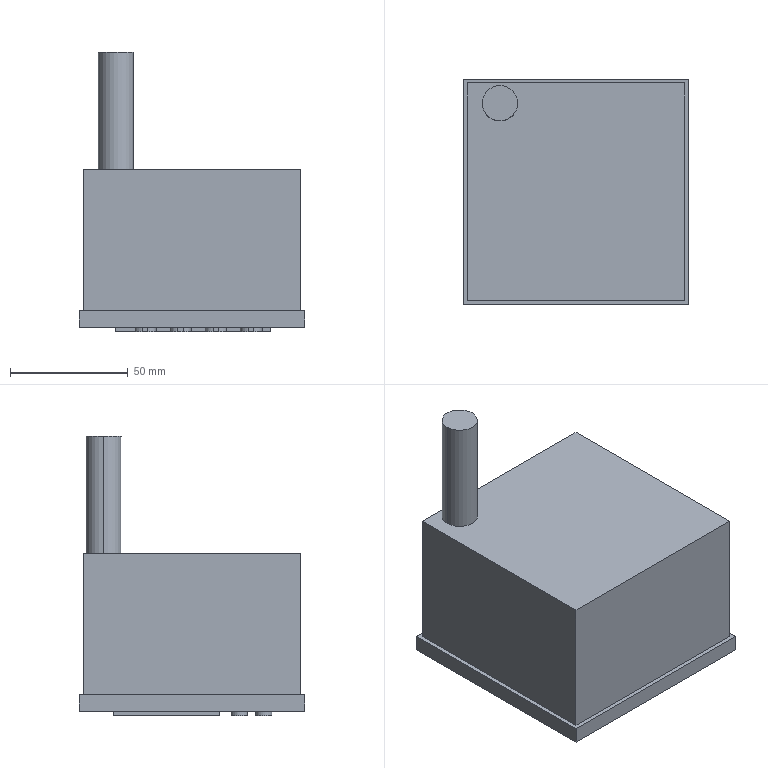Part | STEP file | Shim selection | 1 solid | 67 faces | box 96 x 96 x 119 mm | volume 593520 mm3 | plane 41 | cylinder 26 | commonest cylinder face diameters 6.961 x24 15 x2